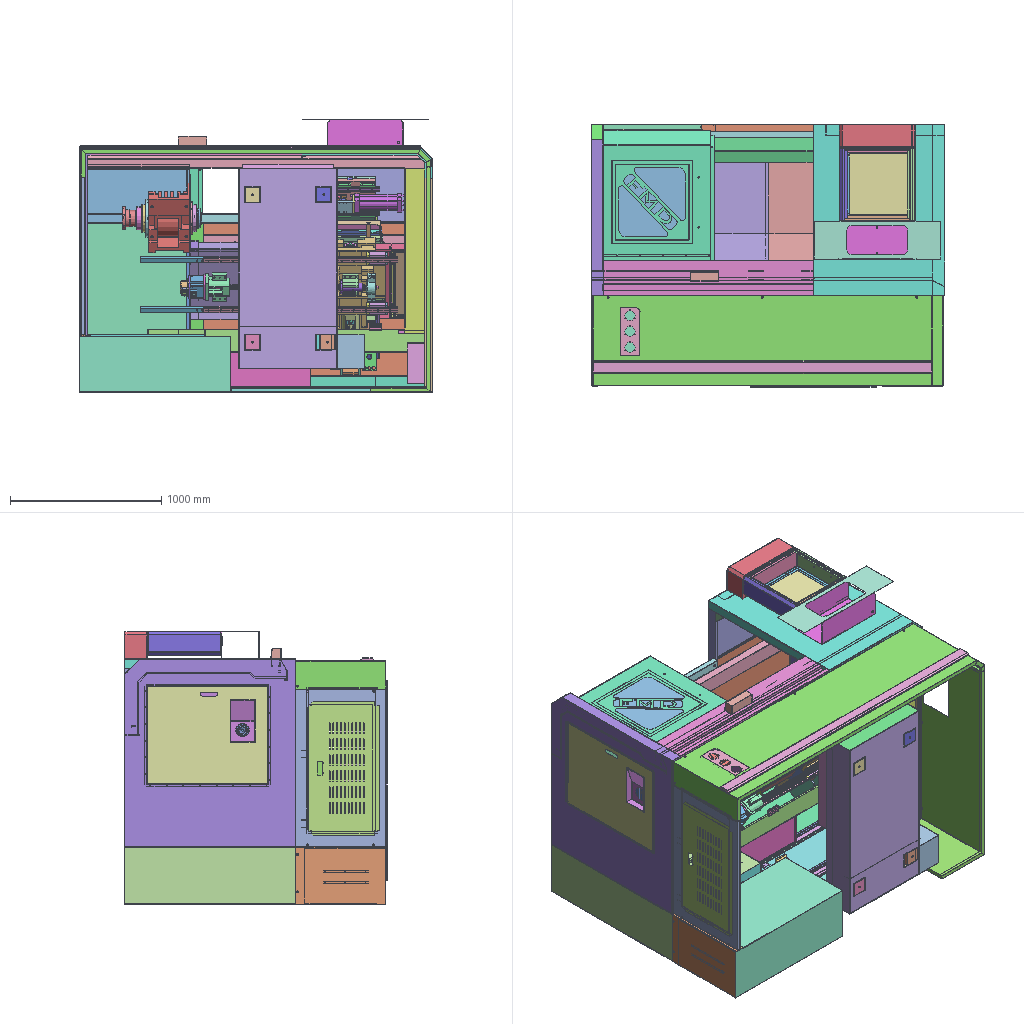Assembly | STEP file | 228 different items | 297 placed | box 2338 x 1737 x 1802 mm
Parts list (item | name | quantity | parent item | size | volume):
1 | 110ST-M04030LFBZ | x1 | in 400MYCV80 Machine Tool Assembly | 130 x 168 x 283 mm | 2271146 mm3
2 | 130ST-M04025LSB | x1 | in 400MYCV80 Machine Tool Assembly | 130 x 176 x 226 mm | 2134855 mm3
3 | 25TAC628B Bearing | x8 | in 400MYCV80 Machine Tool Assembly | 62 x 15 x 62 mm | 31860 mm3
4 | 400V80 Main Carriage | x1 | in 400MYCV80 Machine Tool Assembly | 460 x 660 x 110 mm | 11803093 mm3
5 | 400V80 X-Axis Lead Screw | x1 | in 400MYCV80 Machine Tool Assembly | 32 x 32 x 598 mm | 373661 mm3
6 | 400V80 Z-Axis Lead Screw | x1 | in 400MYCV80 Machine Tool Assembly | 32 x 32 x 1073 mm | 695991 mm3
7 | 400v80 Headstock | x1 | in 400MYCV80 Machine Tool Assembly | 391 x 354.196 x 269 mm | 11825762 mm3
8 | 400v80 Rear Door Filler Piece | x2 | in Rear Closing Plate 1 Assembly, Rear Closing Plate 2 Assembly | 951 x 46.586 x 17 mm | 101104 mm3
9 | 400v80 Rear Door Lower | x1 | in Rear Closing Plate 2 Assembly | 955 x 297 x 20 mm | 675608 mm3
10 | 400v80 Rear Door Upper | x1 | in Rear Closing Plate 1 Assembly | 955 x 627 x 17 mm | 1331439 mm3
11 | 400v80 Rear Panel Filler Piece | x1 | in Right Panel Assembly | 102 x 32 x 80 mm | 20190 mm3
12 | 400v80 Tailstock | x1 | in 400MYCV80 Machine Tool Assembly | 409.5 x 153.533 x 298 mm | 5552005 mm3
13 | 400v80 Tailstock Locating Pin | x2 | in 400MYCV80 Machine Tool Assembly | 30 x 75 x 30 mm | 61563 mm3
14 | 400v80 Water Tank Main Assembly | x1 | in 2 | - | -
15 | 40FDD Lead Screw Nut Seat | x2 | in 400MYCV80 Machine Tool Assembly | 130 x 98.329 x 100 mm | 642509 mm3
16 | 45L X Bearing Seat | x1 | in 400MYCV80 Machine Tool Assembly | 140 x 90 x 50 mm | 231952 mm3
17 | 45L X-Direction Motor Mount | x1 | in 400MYCV80 Machine Tool Assembly | 200 x 130 x 160 mm | 1107999 mm3
18 | 45L Z-Direction Motor Mount | x1 | in 400MYCV80 Machine Tool Assembly | 174 x 130 x 160 mm | 1032339 mm3
19 | 45LFDDC Lead Screw Seat | x1 | in 400MYCV80 Machine Tool Assembly | 87 x 87 x 147 mm | 256572 mm3
20 | 45LFDDC Lead Screw Seat 8M | x1 | in 400MYCV80 Machine Tool Assembly | 91 x 73.5 x 132 mm | 225854 mm3
21 | 45Z Bearing Seat | x1 | in 400MYCV80 Machine Tool Assembly | 199.394 x 100 x 60 mm | 453459 mm3
22 | 46 Belt Pulley | x1 | in 46 Motor Spindle Assembly | 86 x 150 x 150 mm | 425226 mm3
23 | 46 Coil | x1 | in 46 Motor Spindle Main Assembly | 210 x 210 x 185 mm | 3277014 mm3
24 | 46 Spindle Front Sleeve | x1 | in 46 Motor Spindle Assembly | 76 x 220 x 220 mm | 975565 mm3
25 | 46 Spindle Front Sleeve 2 | x1 | in 46 Motor Spindle Assembly | 29 x 178 x 178 mm | 367063 mm3
26 | 46 Spindle Inner Shaft | x1 | in 46 Motor Spindle Assembly | 501 x 133 x 133 mm | 1064151 mm3
27 | 5-Way Oil Manifold | x1 | in 400MYCV80 Machine Tool Assembly | 101.057 x 16 x 91 mm | 41067 mm3
28 | 520 Sliding Door | x1 | in 520 Sliding Door Assembly | 803 x 928 x 391 mm | 1999318 mm3
29 | 7014 Inner Spacer | x1 | in 46 Motor Spindle Assembly | 99 x 99 x 51.5 mm | 71782 mm3
30 | 7014C | x2 | in 46 Motor Spindle Assembly | 20 x 110 x 110 mm | 86450 mm3
31 | 7016 | x3 | in 46 Motor Spindle Assembly | 125 x 125 x 22 mm | 114656 mm3
32 | 7016 Inner Spacer | x1 | in 46 Motor Spindle Assembly | 108 x 108 x 9.5 mm | 39276 mm3
33 | 7016 Nut 2 | x1 | in 46 Motor Spindle Assembly | 105 x 104.847 x 18 mm | 64985 mm3
34 | Aluminium Alloy Bracket | x2 | in 400MYCV80 Machine Tool Assembly | 84 x 16 x 46 mm | 29509 mm3
35 | Box Control Box | x1 | in Control Box Assembly | 502 x 160 x 31.5 mm | 198922 mm3
36 | Brake Resistor Plate | x1 | in Electrical Cabinet Assembly | 184 x 14 x 650 mm | 267329 mm3
37 | Cable Chain Bracket-1 | x1 | in Cable Chain Box Bracket Assembly | 27.758 x 83.881 x 4 mm | 4206 mm3
38 | Cable Chain Bracket_Default SM-FLAT-PATTERN | x1 | in Cable Chain Box Bracket Assembly | 299.33 x 85.981 x 95.1 mm | 199185 mm3
39 | Center Shaft Plate | x1 | in 400V80 Main Guard Assembly | 1167 x 1091 x 25 mm | 650871 mm3
40 | Center Shaft Plate 2 | x1 | in 2 | 1053 x 1022 x 2 mm | 1400799 mm3
41 | Center Shaft Plate Rib | x1 | in 400V80 Main Guard Assembly | 90 x 22 x 736 mm | 186338 mm3
42 | Clamp Frame Weldment 1 | x2 | in Sliding Door Clamp Frame Weldment Assembly | 534 x 25 x 15 mm | 51628 mm3
43 | Clamp Frame Weldment 2 | x2 | in Sliding Door Clamp Frame Weldment Assembly | 25 x 550 x 15 mm | 50877 mm3
44 | Clip | x1 | in 400V80 Main Guard Assembly | 22 x 45 x 12 mm | 1529 mm3
45 | Closing Plate Clip | x4 | in Electrical Cabinet Lower Box Closing Plate Assembly, Rear Closing Plate 2 Assembly | 50 x 18 x 36 mm | 5781 mm3
46 | Connecting Seat | x1 | in 400MYCV80 Machine Tool Assembly | 260 x 40 x 260 mm | 2352118 mm3
47 | Control Box 1 | x1 | in Control Box Assembly | 51 x 160 x 476 mm | 222530 mm3
48 | Control Box 2 | x1 | in Control Box Assembly | 51 x 160 x 476 mm | 211731 mm3
49 | Control Box 3 | x1 | in Control Box Assembly | 502 x 160 x 31.5 mm | 198922 mm3
50 | Control Box Housing | x1 | in 2 | 190 x 69.286 x 70 mm | 74278 mm3
51 | Control Box Inner Spacer | x1 | in Control Box Assembly | 470.879 x 472 x 2 mm | 126938 mm3
52 | Control Box Lower Base 1 | x1 | in Control Box Lower Assembly 1 | 498 x 178 x 250 mm | 589659 mm3
53 | Control Box Lower Base 2 | x1 | in Control Box Lower Assembly 1 | 832.569 x 2 x 250 mm | 265061 mm3
54 | Control Box Rear Closing Plate | x1 | in Control Box Assembly | 433 x 435 x 2 mm | 376395 mm3
55 | Control Box Top Cover | x1 | in Control Box Upper Assembly 1 | 459 x 157 x 2 mm | 143288 mm3
56 | Control Box Upper 1 | x1 | in Control Box Upper Assembly 1 | 502 x 150 x 180.5 mm | 475305 mm3
57 | Control Box Upper 3 | x1 | in Control Box Upper Assembly 1 | 482 x 168.4 x 2 mm | 45264 mm3
58 | DT-012 | x1 | in 400MYCV80 Machine Tool Assembly | 53 x 38 x 400 mm | 103503 mm3
59 | Door Clip | x1 | in 400V80 Main Guard Assembly | 25 x 19 x 2 mm | 893.451 mm3
60 | Electrical Cabinet 1 | x1 | in Electrical Cabinet Assembly | 832 x 1130 x 380 mm | 3955545 mm3
61 | Electrical Cabinet 2 | x1 | in Electrical Cabinet Assembly | 828 x 78 x 378 mm | 762303 mm3
62 | Electrical Cabinet 3 | x1 | in Electrical Cabinet Assembly | 828 x 78 x 378 mm | 749579 mm3
63 | Electrical Cabinet 4 | x1 | in 400V80 Main Guard Assembly | 18 x 38 x 787 mm | 98709 mm3
64 | Electrical Cabinet 5 | x1 | in 400V80 Main Guard Assembly | 352 x 38 x 18 mm | 43368 mm3
65 | Electrical Cabinet Base Plate | x1 | in 2 | 680 x 985 x 20 mm | 1454613 mm3
66 | Electrical Cabinet Base Plate Rib | x2 | in Electrical Cabinet Assembly | 660 x 30 x 25 mm | 98224 mm3
67 | Electrical Cabinet Door | x1 | in 2 | 708 x 1006 x 21 mm | 1538935 mm3
68 | Electrical Cabinet Lower Box Assembly | x1 | in 2 | - | -
69 | Electrical Cabinet Lower Box Closing Plate | x1 | in Electrical Cabinet Lower Box Closing Plate Assembly | 876 x 479.5 x 19.5 mm | 704453 mm3
70 | Encoder | x1 | in 46 Motor Spindle Assembly | 182 x 182 x 44 mm | 482174 mm3
71 | End Cover | x1 | in 400MYCV80 Machine Tool Assembly | 90 x 90 x 15 mm | 46704 mm3
72 | FJ1020 Floating Joint | x1 | in 400MYCV80 Machine Tool Assembly | 102 x 53 x 53 mm | 114072 mm3
73 | Front Base Frame | x1 | in 400V80 Main Guard Assembly | 2334 x 83.033 x 138 mm | 848369 mm3
74 | Front Left Filler Piece | x1 | in 400V80 Main Guard Assembly | 20 x 57.062 x 114.125 mm | 10515 mm3
75 | Front Panel | x1 | in Front Panel Assembly | 2314 x 597 x 206.5 mm | 2666967 mm3
76 | Front Plate | x1 | in 400V80 Main Guard Assembly | 1390 x 268 x 55 mm | 1100627 mm3
77 | Front Plate-1 | x1 | in 400V80 Main Guard Assembly | 20 x 45 x 2 mm | 1800 mm3
78 | Front Trim Panel | x1 | in 2 | 85 x 20 x 2241 mm | 442724 mm3
79 | Guard Rib | x1 | in 400V80 Main Guard Assembly | 30 x 673.333 x 80 mm | 175185 mm3
80 | Guard Rib 2 | x1 | in 400V80 Main Guard Assembly | 30 x 290.188 x 502.62 mm | 129712 mm3
81 | Guard Rib 3 | x1 | in 400V80 Main Guard Assembly | 30 x 129.355 x 80 mm | 28343 mm3
82 | Guard Stiffening Rib | x1 | in 400V80 Main Guard Assembly | 60 x 30 x 1408 mm | 244838 mm3
83 | HAK32080 Outline | x1 | in 400MYCV80 Machine Tool Assembly | 283 x 275 x 483.5 mm | 14482459 mm3
84 | HGH30_2 | x4 | in 400MYCV80 Machine Tool Assembly | 60 x 39.001 x 97.4 mm | 169047 mm3
85 | HGR30_1 | x2 | in 400MYCV80 Machine Tool Assembly | 28 x 26 x 790 mm | 457058 mm3
86 | HWH35HA Slider Block | x4 | in 400MYCV80 Machine Tool Assembly | 70 x 47.5 x 138.2 mm | 358074 mm3
87 | HWH35HA1080 | x2 | in 400MYCV80 Machine Tool Assembly | 1280 x 29 x 34 mm | 1077935 mm3
88 | Hydraulic Cylinder Bracket | x1 | in 400MYCV80 Machine Tool Assembly | 110 x 30 x 400 mm | 265743 mm3
89 | Hydraulic Cylinder Connecting Bracket | x1 | in 400MYCV80 Machine Tool Assembly | 70 x 60 x 75 mm | 78715 mm3
90 | Hydraulic Cylinder Fixing Bracket | x1 | in 400MYCV80 Machine Tool Assembly | 140 x 110 x 90 mm | 268205 mm3
91 | Hydraulic Cylinder Rod 2 | x1 | in 400MYCV80 Machine Tool Assembly | 50 x 50 x 290 mm | 385630 mm3
92 | Inner Lining Plate | x1 | in 400V80 Main Guard Assembly | 728 x 988 x 415.5 mm | 2061913 mm3
93 | Left Cover Plate | x1 | in 400MYCV80 Machine Tool Assembly | 45 x 120 x 260 mm | 111585 mm3
94 | Left Door | x1 | in Left Door Assembly | 645 x 795 x 21 mm | 1111473 mm3
95 | Left Door Filler Piece A | x1 | in Left Door Assembly | 280 x 165 x 51.682 mm | 136395 mm3
96 | Left Door Frame 1 | x2 | in Left Door Frame Weldment Assembly | 22 x 804 x 28 mm | 75069 mm3
97 | Left Door Frame 2 | x2 | in Left Door Frame Weldment Assembly | 650 x 33 x 22 mm | 65954 mm3
98 | Left Side Panel | x1 | in Left Side Panel Assembly | 28.5 x 597 x 1036 mm | 608718 mm3
99 | Left Side Panel Closing Plate | x1 | in Left Side Panel Door Assembly | 885.969 x 475.969 x 1.5 mm | 584980 mm3
100 | Left Side Panel Frame Left | x1 | in Left Side Panel Frame Assembly | 26.5 x 455 x 20 mm | 29759 mm3
101 | Left Side Panel Frame Lower | x1 | in Left Side Panel Frame Assembly | 940 x 13.5 x 15 mm | 37314 mm3
102 | Left Side Panel Frame Right | x1 | in Left Side Panel Frame Assembly | 26.5 x 455 x 20 mm | 29759 mm3
103 | Left Side Panel Frame Upper | x1 | in Left Side Panel Frame Assembly | 26.5 x 20 x 964 mm | 62237 mm3
104 | Left Side Plate | x1 | in 400V80 Main Guard Assembly | 1240 x 1166 x 80 mm | 2225373 mm3
105 | Left Side Plate Filler Piece | x1 | in 400V80 Main Guard Assembly | 502.056 x 112.482 x 80 mm | 112790 mm3
106 | Limit Switch | x2 | in 400MYCV80 Machine Tool Assembly | 55 x 51 x 77 mm | 154232 mm3
107 | Lock Nut | x1 | in 400MYCV80 Machine Tool Assembly | 52 x 52 x 18 mm | 20909 mm3
108 | Motor Cover | x2 | in 400MYCV80 Machine Tool Assembly | 113 x 100 x 2 mm | 22277 mm3
109 | Oil Filler Tank | x1 | in Oil Filler Tank Assembly | 267 x 305 x 168.5 mm | 340188 mm3
110 | Oil Filler Tank Closing Plate | x1 | in Oil Filler Tank Assembly | 166.5 x 301 x 2 mm | 99472 mm3
111 | Oil Filler Tank Closing Plate 1 | x1 | in Oil Filler Tank Assembly | 166.5 x 301 x 2 mm | 100233 mm3
112 | Oil Pressure Gauge Panel | x1 | in Front Panel Assembly | 148.239 x 338.239 x 2 mm | 76534 mm3
113 | Oil Pressure Gauge Panel Arc | x1 | in Front Panel Assembly | 30 x 30 x 8 mm | 728.849 mm3
114 | Quick-Release Clip | x2 | in Left Side Panel Door Assembly | 50 x 18 x 36 mm | 5781 mm3
115 | Rear Base Frame | x1 | in 400V80 Main Guard Assembly | 1881 x 75 x 152 mm | 779806 mm3
116 | Rear Base Frame-1 | x3 | in 400V80 Main Guard Assembly | 35 x 23 x 2 mm | 1285 mm3
117 | Rear Base Frame-2 | x1 | in 400V80 Main Guard Assembly | 228 x 273 x 25 mm | 168843 mm3
118 | Rear Closing Plate Door Frame Left | x1 | in Rear Closing Plate Door Frame Assembly | 32 x 650 x 22 mm | 74925 mm3
119 | Rear Closing Plate Door Frame Lower 1 | x1 | in Rear Closing Plate Door Frame Assembly | 959 x 20 x 16 mm | 63977 mm3
120 | Rear Closing Plate Door Frame Right | x1 | in Rear Closing Plate Door Frame Assembly | 30 x 650.24 x 22 mm | 72183 mm3
121 | Rear Closing Plate Door Frame Upper | x1 | in Rear Closing Plate Door Frame Assembly | 963 x 30 x 22 mm | 107174 mm3
122 | Rear Closing Plate Frame Lower 1 | x1 | in Rear Closing Plate Frame Assembly | 963 x 20 x 22 mm | 74999 mm3
123 | Rear Closing Plate Frame Lower 2 | x1 | in Rear Closing Plate Frame Assembly | 959 x 20 x 16 mm | 63977 mm3
124 | Rear Closing Plate Frame Lower 3 | x1 | in Rear Closing Plate Frame Assembly | 20 x 320 x 20 mm | 23444 mm3
125 | Rear Closing Plate Frame Lower 4 | x1 | in Rear Closing Plate Frame Assembly | 20 x 320 x 22 mm | 25233 mm3
126 | Rear Closing Plate Handle | x1 | in Rear Closing Plate 1 Assembly | 123 x 62.38 x 25 mm | 20088 mm3
127 | Rear Door Handle 80 | x3 | in Electrical Cabinet Lower Box Closing Plate Assembly, Rear Closing Plate 2 Assembly | 83 x 40 x 25 mm | 11260 mm3
128 | Rear End Cover | x1 | in 46 Motor Spindle Assembly | 250 x 250 x 42 mm | 1311495 mm3
129 | Rear End Cover 2 | x1 | in 46 Motor Spindle Assembly | 182 x 182 x 21 mm | 315087 mm3
130 | Rear Panel Middle | x1 | in 2 | 923 x 240 x 26 mm | 474595 mm3
131 | Rear Plate | x1 | in 400V80 Main Guard Assembly | 1504 x 1166 x 40 mm | 1850918 mm3
132 | Right Base Frame | x1 | in 400V80 Main Guard Assembly | 185 x 48 x 1095 mm | 500987 mm3
133 | Right Cover Plate | x1 | in 400MYCV80 Machine Tool Assembly | 20 x 120 x 260 mm | 79765 mm3
134 | Right Door Frame 1 | x1 | in Right Door Frame Weldment Assembly | 25 x 764 x 35 mm | 95446 mm3
135 | Right Door Frame 2 | x1 | in Right Door Frame Weldment Assembly | 25 x 764 x 35 mm | 95443 mm3
136 | Right Door Frame 3 | x1 | in Right Door Frame Weldment Assembly | 580 x 35 x 25 mm | 72212 mm3
137 | Right Door Frame 4 | x1 | in Right Door Frame Weldment Assembly | 580 x 45 x 25 mm | 81646 mm3
138 | Right Door Upper Clamp Rib Weldment | x2 | in Right Small Door Frame Weldment Assembly | 403 x 14 x 25 mm | 35999 mm3
139 | Right Front | x1 | in 400V80 Main Guard Assembly | 868 x 1166 x 207 mm | 2658932 mm3
140 | Right Side Panel | x1 | in Right Panel Assembly | 1489 x 597 x 416 mm | 1815164 mm3
141 | Right Side Plate | x1 | in 400V80 Main Guard Assembly | 55 x 1166 x 1423 mm | 2424332 mm3
142 | Right Small Door | x1 | in Right Small Door Assembly | 22 x 745 x 575 mm | 822578 mm3
143 | Right Small Door Clamp Frame 1 | x2 | in Right Small Door Clamp Frame Assembly | 376 x 35 x 15 mm | 23799 mm3
144 | Right Small Door Clamp Frame 2 | x2 | in Right Small Door Clamp Frame Assembly | 35 x 403 x 15 mm | 25676 mm3
145 | Right Small Door Clamp Frame Weldment 1 | x2 | in Right Small Door Frame Weldment Assembly | 372 x 25 x 14 mm | 33377 mm3
146 | Right Small Door Splash Plate | x1 | in Right Small Door Assembly | 29.5 x 38.166 x 504 mm | 40648 mm3
147 | Rotating Shaft | x2 | in 2 | 95 x 18 x 95 mm | 39641 mm3
148 | Sliding Door Lower Rail | x1 | in 400V80 Main Guard Assembly | 24 x 61.13 x 1420 mm | 280395 mm3
149 | Sliding Door Lower Rail Weldment | x1 | in 400V80 Main Guard Assembly | 46 x 60 x 1467 mm | 339096 mm3
150 | Sliding Door Lower Rail Weldment-1 | x1 | in 400V80 Main Guard Assembly | 26 x 56 x 2 mm | 2832 mm3
151 | Sliding Door Spacer Block | x1 | in 520 Sliding Door Assembly | 690 x 10 x 35 mm | 68950 mm3
152 | Sliding Door Upper Rail | x1 | in 400V80 Main Guard Assembly | 60 x 40 x 1467 mm | 413342 mm3
153 | Spindle Inner Ring | x1 | in 46 Motor Spindle Assembly | 135 x 135 x 151 mm | 1278709 mm3
154 | Spindle Inner Spacer | x2 | in 46 Motor Spindle Assembly | 82 x 82 x 23 mm | 27819 mm3
155 | Spindle Rear Nut | x1 | in 46 Motor Spindle Assembly | 91.8 x 91.8 x 27.6 mm | 66941 mm3
156 | T Slider Block | x16 | in xzz-001 Assembly, xzz-002 Assembly, xzz-003 Assembly, zh001 Assembly, zh002 Assembly, zp001 Assembly, zp002 Assembly | 60 x 38 x 9 mm | 10054 mm3
157 | TX-003 | x1 | in TX 001 Assembly | 395 x 279 x 220.81 mm | 327084 mm3
158 | TX-003-1 | x1 | in TX 001 Assembly | 722 x 399 x 15 mm | 342555 mm3
159 | TX-005 | x1 | in TX 001 Assembly | 505.19 x 399 x 15 mm | 294466 mm3
160 | TX-01-1 | x1 | in TX 001 Assembly | 724 x 82 x 395 mm | 558409 mm3
161 | Tail End Cover | x1 | in 400MYCV80 Machine Tool Assembly | 90 x 90 x 75 mm | 127582 mm3
162 | Tailstock Sleeve | x1 | in 400MYCV80 Machine Tool Assembly | 60 x 60 x 310 mm | 687459 mm3
163 | Telescopic Hydraulic Cylinder | x1 | in 400MYCV80 Machine Tool Assembly | 90 x 90 x 365 mm | 1281349 mm3
164 | Telescopic Rod 2 | x1 | in 400MYCV80 Machine Tool Assembly | 30 x 30 x 300 mm | 200246 mm3
165 | Top Cover 1 | x1 | in 400V80 Main Guard Assembly | 1618 x 85 x 1128 mm | 3307611 mm3
166 | Top Cover 2 | x1 | in 400V80 Main Guard Assembly | 868 x 66 x 502.5 mm | 820735 mm3
167 | Top Cover 3 | x1 | in 400V80 Main Guard Assembly | 728 x 97 x 738 mm | 1251055 mm3
168 | Transformer Cover 1 | x1 | in 400V80 Main Guard Assembly | 700 x 20 x 263 mm | 434709 mm3
169 | Trunking 1 | x1 | in 400V80 Main Guard Assembly | 1504 x 70 x 106 mm | 380057 mm3
170 | Trunking 2 | x1 | in 400V80 Main Guard Assembly | 90 x 70 x 735 mm | 175454 mm3
171 | Trunking 3 | x1 | in 400V80 Main Guard Assembly | 1.5 x 173.707 x 1387 mm | 353324 mm3
172 | Trunking 4 | x1 | in 400V80 Main Guard Assembly | 785 x 122.735 x 70 mm | 203743 mm3
173 | Trunking Cover 2 Spacer Plate | x3 | in 400V80 Main Guard Assembly | 716 x 97.011 x 1.5 mm | 41639 mm3
174 | Trunking Light 5 | x1 | in 400V80 Main Guard Assembly | 1408 x 58 x 107 mm | 462641 mm3
175 | Trunking Light 6 | x1 | in 400V80 Main Guard Assembly | 65 x 800 x 35 mm | 157112 mm3
176 | Trunking Spacer Plate | x2 | in 400V80 Main Guard Assembly | 420 x 104 x 2 mm | 38692 mm3
177 | Trunking Spacer Plate 2 | x1 | in 400V80 Main Guard Assembly | 420 x 90 x 2 mm | 21986 mm3
178 | Turret 32080 Tool Holder Base Plate | x1 | in 400MYCV80 Machine Tool Assembly | 152 x 210 x 29 mm | 892737 mm3
179 | Turret Tool Holder Base Plate | x1 | in 400MYCV80 Machine Tool Assembly | 348 x 60 x 410 mm | 5898347 mm3
180 | Wheel Fixing Plate | x1 | in 520 Sliding Door Assembly | 780 x 107 x 37 mm | 186121 mm3
181 | X Limit Switch Bracket | x1 | in 400MYCV80 Machine Tool Assembly | 25 x 30 x 15 mm | 2701 mm3
182 | X Motor Cover 1 | x1 | in X Motor Cover Assembly | 135 x 230 x 260 mm | 237291 mm3
183 | X Motor Cover 1-1 | x1 | in X Motor Cover Assembly | 132 x 228.5 x 15 mm | 47221 mm3
184 | X Travel Bracket | x1 | in 400MYCV80 Machine Tool Assembly | 60 x 30 x 380 mm | 85607 mm3
185 | X Travel Bracket 2 | x1 | in 400MYCV80 Machine Tool Assembly | 100 x 50 x 60 mm | 23920 mm3
186 | X-Axis 28 Guide Rail | x2 | in 400MYCV80 Machine Tool Assembly | 28 x 449.72 x 449.72 mm | 422177 mm3
187 | X-Axis 28 Guide Rail Slider Block | x4 | in 400MYCV80 Machine Tool Assembly | 60 x 95.035 x 95.035 mm | 165273 mm3
188 | X-Axis Clamp Block | x2 | in 400MYCV80 Machine Tool Assembly | 19.179 x 10 x 96 mm | 16808 mm3
189 | X-Axis Clamp Block 1 | x1 | in 400MYCV80 Machine Tool Assembly | 120 x 10 x 10 mm | 12000 mm3
190 | YCR72x1.5 Radial Lock Nut | x1 | in 46 Motor Spindle Assembly | 95 x 18 x 94.809 mm | 50193 mm3
191 | Z Travel Bracket | x1 | in 400MYCV80 Machine Tool Assembly | 57.598 x 65.981 x 60 mm | 17695 mm3
192 | Z-Direction Cover Plate | x1 | in 2 | 1571 x 215.846 x 58.382 mm | 647341 mm3
193 | xzz-001 | x1 | in xzz-001 Assembly | 404 x 100 x 100 mm | 122161 mm3
194 | xzz-001-1 | x1 | in xzz-001 Assembly | 400 x 78 x 2 mm | 34179 mm3
195 | xzz-001-1-01 | x2 | in xzz-001 Assembly | 42 x 25 x 2 mm | 1694 mm3
196 | xzz-001-2 | x1 | in xzz-001 Assembly | 404 x 120 x 2 mm | 40299 mm3
197 | xzz-002 | x1 | in xzz-002 Assembly | 392 x 91.5 x 87 mm | 101252 mm3
198 | xzz-002-1 | x1 | in xzz-002 Assembly | 397.4 x 76.7 x 2 mm | 32215 mm3
199 | xzz-003 | x1 | in xzz-003 Assembly | 380 x 83 x 80 mm | 88406 mm3
200 | xzz-003-1 | x1 | in xzz-003 Assembly | 385.4 x 70.7 x 2 mm | 25743 mm3
201 | xzz-004 | x1 | in xzz-004 Assembly | 368 x 74.5 x 72 mm | 73899 mm3
202 | xzz-004-1 | x1 | in xzz-004 Assembly | 373.4 x 64.7 x 2 mm | 19566 mm3
203 | xzz-004-2 | x1 | in xzz-005 Assembly | 356 x 70 x 2 mm | 39282 mm3
204 | xzz-005 | x1 | in xzz-005 Assembly | 356 x 66 x 69 mm | 66855 mm3
205 | xzz-005-1 | x1 | in xzz-005 Assembly | 361.4 x 58.7 x 2 mm | 18757 mm3
206 | xzz-Auxiliary Guide Rail | x2 | in 400MYCV80 Machine Tool Assembly | 28 x 26 x 125 mm | 88103 mm3
207 | zh001 | x1 | in zh001 Assembly | 840.386 x 564.059 x 459.75 mm | 808463 mm3
208 | zh001-1 | x1 | in zh001 Assembly | 827.736 x 568.01 x 2 mm | 95326 mm3
209 | zh002 | x1 | in zh002 Assembly | 827.795 x 553.29 x 210 mm | 501438 mm3
210 | zh002-1 | x1 | in zh002 Assembly | 824.943 x 563.765 x 2 mm | 93562 mm3
211 | zh003 | x1 | in zh003 Assembly | 815.204 x 542.52 x 205 mm | 479740 mm3
212 | zh003-1 | x1 | in zh003 Assembly | 812.643 x 554.564 x 2 mm | 76512 mm3
213 | zh004 | x1 | in zh004 Assembly | 802.614 x 531.751 x 210 mm | 477513 mm3
214 | zh004-1 | x1 | in zh004 Assembly | 804.508 x 546.826 x 2 mm | 67085 mm3
215 | zh004-2 | x1 | in zh005-2 | 823.438 x 570.114 x 3 mm | 212618 mm3
216 | zh005 | x1 | in zh005-2 | 791.755 x 520.982 x 214 mm | 471579 mm3
217 | zh005-1 | x1 | in zh005-2 | 796.98 x 541.285 x 2 mm | 53222 mm3
218 | zq Auxiliary Guide Rail | x2 | in 400MYCV80 Machine Tool Assembly | 34 x 29 x 420 mm | 407406 mm3
219 | zq001 | x1 | in zp001 Assembly | 840.386 x 564.059 x 655.75 mm | 1280382 mm3
220 | zq001-1 | x1 | in zp001 Assembly | 827.736 x 568.376 x 2 mm | 90659 mm3
221 | zq001-2 | x1 | in zp001 Assembly | 835.227 x 571.502 x 2 mm | 101233 mm3
222 | zq002 | x1 | in zp002 Assembly | 853.41 x 576.829 x 440 mm | 1105453 mm3
223 | zq002-1 | x1 | in zp002 Assembly | 845.991 x 579.972 x 2 mm | 116517 mm3
224 | zzf001 | x1 | in zzf-001 Assembly | 488.4 x 86.155 x 44.301 mm | 95015 mm3
225 | zzf001-1 | x1 | in zzf-001 Assembly | 60 x 401.094 x 42.5 mm | 75314 mm3
226 | zzf001-2 | x1 | in zzf-001 Assembly | 60 x 401.094 x 42.5 mm | 75314 mm3
227 | zzh001 | x1 | in zzh001 Assembly | 53 x 587.725 x 864.748 mm | 128593 mm3
228 | zzh002 | x1 | in zzh001 Assembly | 3 x 648.349 x 935.758 mm | 197054 mm3